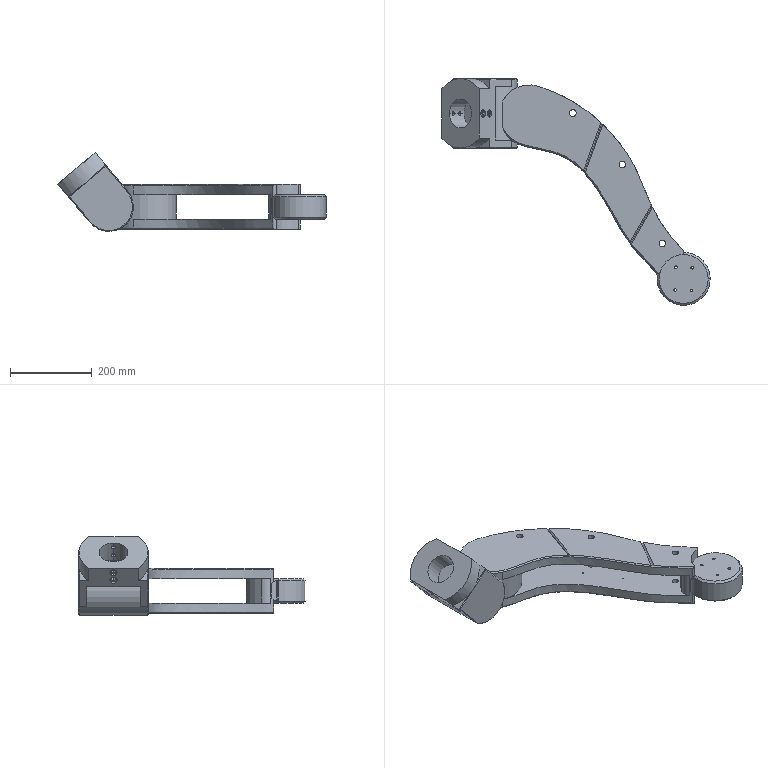Part | SolidWorks | features MirrorStock 1 | 1 solid | 136 faces | box 657.517 x 555 x 192.791 mm | volume 7755775 mm3 | cylinder 71 | plane 43 | cone 15 | spline 7 | commonest cylinder face diameters 16 x12 6.6 x8 10.2 x8 18 x8 10 x6 40 x5